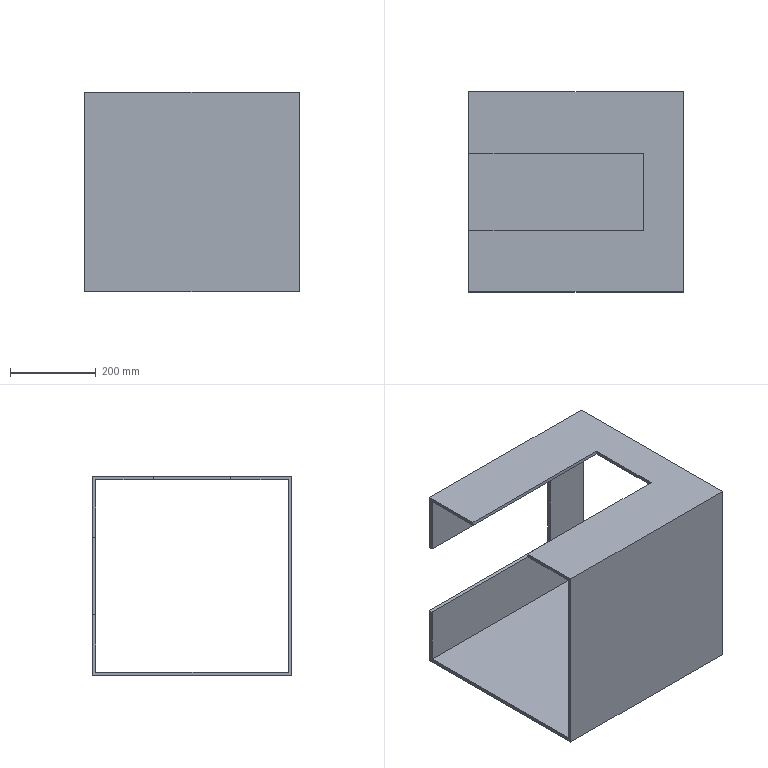Part | SolidWorks | features Cut 2, DeleteBody 1, Extrusion 1, MoveCopyBody 1, Stock 1 | 1 solid | 17 faces | box 500 x 466 x 466 mm | volume 6178880 mm3 | plane 17
STEP:
#1=CARTESIAN_POINT('',(0.,-90.,233.));
#2=VERTEX_POINT('',#1);
#3=CARTESIAN_POINT('',(0.,-233.,233.));
#4=VERTEX_POINT('',#3);
#5=CARTESIAN_POINT('',(0.,233.,233.));
#6=DIRECTION('',(0.,-1.,0.));
#7=VECTOR('',#6,1000.);
#8=LINE('',#5,#7);
#9=EDGE_CURVE('',#2,#4,#8,.T.);
#10=ORIENTED_EDGE('',*,*,#9,.F.);
#11=CARTESIAN_POINT('',(0.,-90.,225.));
#12=VERTEX_POINT('',#11);
#13=CARTESIAN_POINT('',(0.,-90.,98.286));
#14=DIRECTION('',(0.,0.,1.));
#15=VECTOR('',#14,1000.);
#16=LINE('',#13,#15);
#17=EDGE_CURVE('',#12,#2,#16,.T.);
#18=ORIENTED_EDGE('',*,*,#17,.F.);
#19=CARTESIAN_POINT('',(0.,-225.,225.));
#20=VERTEX_POINT('',#19);
#21=CARTESIAN_POINT('',(0.,225.,225.));
#22=DIRECTION('',(0.,-1.,0.));
#23=VECTOR('',#22,1000.);
#24=LINE('',#21,#23);
#25=EDGE_CURVE('',#12,#20,#24,.T.);
#26=ORIENTED_EDGE('',*,*,#25,.T.);
#27=CARTESIAN_POINT('',(0.,-225.,-225.));
#28=VERTEX_POINT('',#27);
#29=CARTESIAN_POINT('',(0.,-225.,225.));
#30=DIRECTION('',(0.,0.,-1.));
#31=VECTOR('',#30,1000.);
#32=LINE('',#29,#31);
#33=EDGE_CURVE('',#20,#28,#32,.T.);
#34=ORIENTED_EDGE('',*,*,#33,.T.);
#35=CARTESIAN_POINT('',(0.,225.,-225.));
#36=VERTEX_POINT('',#35);
#37=CARTESIAN_POINT('',(0.,225.,-225.));
#38=DIRECTION('',(0.,1.,0.));
#39=VECTOR('',#38,1000.);
#40=LINE('',#37,#39);
#41=EDGE_CURVE('',#28,#36,#40,.T.);
#42=ORIENTED_EDGE('',*,*,#41,.T.);
#43=CARTESIAN_POINT('',(0.,225.,-90.));
#44=VERTEX_POINT('',#43);
#45=CARTESIAN_POINT('',(0.,225.,225.));
#46=DIRECTION('',(0.,0.,1.));
#47=VECTOR('',#46,1000.);
#48=LINE('',#45,#47);
#49=EDGE_CURVE('',#36,#44,#48,.T.);
#50=ORIENTED_EDGE('',*,*,#49,.T.);
#51=CARTESIAN_POINT('',(0.,233.,-90.));
#52=VERTEX_POINT('',#51);
#53=CARTESIAN_POINT('',(0.,0.,-90.));
#54=DIRECTION('',(0.,1.,0.));
#55=VECTOR('',#54,1000.);
#56=LINE('',#53,#55);
#57=EDGE_CURVE('',#44,#52,#56,.T.);
#58=ORIENTED_EDGE('',*,*,#57,.T.);
#59=CARTESIAN_POINT('',(0.,233.,-233.));
#60=VERTEX_POINT('',#59);
#61=CARTESIAN_POINT('',(0.,233.,233.));
#62=DIRECTION('',(0.,0.,1.));
#63=VECTOR('',#62,1000.);
#64=LINE('',#61,#63);
#65=EDGE_CURVE('',#60,#52,#64,.T.);
#66=ORIENTED_EDGE('',*,*,#65,.F.);
#67=CARTESIAN_POINT('',(0.,-233.,-233.));
#68=VERTEX_POINT('',#67);
#69=CARTESIAN_POINT('',(0.,233.,-233.));
#70=DIRECTION('',(0.,1.,0.));
#71=VECTOR('',#70,1000.);
#72=LINE('',#69,#71);
#73=EDGE_CURVE('',#68,#60,#72,.T.);
#74=ORIENTED_EDGE('',*,*,#73,.F.);
#75=CARTESIAN_POINT('',(0.,-233.,233.));
#76=DIRECTION('',(0.,0.,-1.));
#77=VECTOR('',#76,1000.);
#78=LINE('',#75,#77);
#79=EDGE_CURVE('',#4,#68,#78,.T.);
#80=ORIENTED_EDGE('',*,*,#79,.F.);
#81=EDGE_LOOP('',(#10,#18,#26,#34,#42,#50,#58,#66,#74,#80));
#82=FACE_OUTER_BOUND('',#81,.T.);
#83=CARTESIAN_POINT('',(0.,0.,0.));
#84=DIRECTION('',(1.,0.,0.));
#85=DIRECTION('',(0.,0.,-1.));
#86=AXIS2_PLACEMENT_3D('',#83,#84,#85);
#87=PLANE('',#86);
#88=ADVANCED_FACE('',(#82),#87,.F.);
#89=CARTESIAN_POINT('',(500.,-233.,-233.));
#90=VERTEX_POINT('',#89);
#91=CARTESIAN_POINT('',(500.,233.,-233.));
#92=VERTEX_POINT('',#91);
#93=CARTESIAN_POINT('',(500.,233.,-233.));
#94=DIRECTION('',(0.,1.,0.));
#95=VECTOR('',#94,1000.);
#96=LINE('',#93,#95);
#97=EDGE_CURVE('',#90,#92,#96,.T.);
#98=ORIENTED_EDGE('',*,*,#97,.T.);
#99=CARTESIAN_POINT('',(500.,233.,233.));
#100=VERTEX_POINT('',#99);
#101=CARTESIAN_POINT('',(500.,233.,233.));
#102=DIRECTION('',(0.,0.,1.));
#103=VECTOR('',#102,1000.);
#104=LINE('',#101,#103);
#105=EDGE_CURVE('',#92,#100,#104,.T.);
#106=ORIENTED_EDGE('',*,*,#105,.T.);
#107=CARTESIAN_POINT('',(500.,-233.,233.));
#108=VERTEX_POINT('',#107);
#109=CARTESIAN_POINT('',(500.,233.,233.));
#110=DIRECTION('',(0.,-1.,0.));
#111=VECTOR('',#110,1000.);
#112=LINE('',#109,#111);
#113=EDGE_CURVE('',#100,#108,#112,.T.);
#114=ORIENTED_EDGE('',*,*,#113,.T.);
#115=CARTESIAN_POINT('',(500.,-233.,233.));
#116=DIRECTION('',(0.,0.,-1.));
#117=VECTOR('',#116,1000.);
#118=LINE('',#115,#117);
#119=EDGE_CURVE('',#108,#90,#118,.T.);
#120=ORIENTED_EDGE('',*,*,#119,.T.);
#121=EDGE_LOOP('',(#98,#106,#114,#120));
#122=FACE_OUTER_BOUND('',#121,.T.);
#123=CARTESIAN_POINT('',(500.,225.,-225.));
#124=VERTEX_POINT('',#123);
#125=CARTESIAN_POINT('',(500.,225.,225.));
#126=VERTEX_POINT('',#125);
#127=CARTESIAN_POINT('',(500.,225.,225.));
#128=DIRECTION('',(0.,0.,1.));
#129=VECTOR('',#128,1000.);
#130=LINE('',#127,#129);
#131=EDGE_CURVE('',#124,#126,#130,.T.);
#132=ORIENTED_EDGE('',*,*,#131,.F.);
#133=CARTESIAN_POINT('',(500.,-225.,-225.));
#134=VERTEX_POINT('',#133);
#135=CARTESIAN_POINT('',(500.,225.,-225.));
#136=DIRECTION('',(0.,1.,0.));
#137=VECTOR('',#136,1000.);
#138=LINE('',#135,#137);
#139=EDGE_CURVE('',#134,#124,#138,.T.);
#140=ORIENTED_EDGE('',*,*,#139,.F.);
#141=CARTESIAN_POINT('',(500.,-225.,225.));
#142=VERTEX_POINT('',#141);
#143=CARTESIAN_POINT('',(500.,-225.,225.));
#144=DIRECTION('',(0.,0.,-1.));
#145=VECTOR('',#144,1000.);
#146=LINE('',#143,#145);
#147=EDGE_CURVE('',#142,#134,#146,.T.);
#148=ORIENTED_EDGE('',*,*,#147,.F.);
#149=CARTESIAN_POINT('',(500.,225.,225.));
#150=DIRECTION('',(0.,-1.,0.));
#151=VECTOR('',#150,1000.);
#152=LINE('',#149,#151);
#153=EDGE_CURVE('',#126,#142,#152,.T.);
#154=ORIENTED_EDGE('',*,*,#153,.F.);
#155=EDGE_LOOP('',(#132,#140,#148,#154));
#156=FACE_BOUND('',#155,.T.);
#157=CARTESIAN_POINT('',(500.,0.,0.));
#158=DIRECTION('',(1.,0.,0.));
#159=DIRECTION('',(0.,0.,-1.));
#160=AXIS2_PLACEMENT_3D('',#157,#158,#159);
#161=PLANE('',#160);
#162=ADVANCED_FACE('',(#122,#156),#161,.T.);
#163=CARTESIAN_POINT('',(0.,225.,225.));
#164=VERTEX_POINT('',#163);
#165=CARTESIAN_POINT('',(0.,90.,225.));
#166=VERTEX_POINT('',#165);
#167=CARTESIAN_POINT('',(0.,225.,225.));
#168=DIRECTION('',(0.,-1.,0.));
#169=VECTOR('',#168,1000.);
#170=LINE('',#167,#169);
#171=EDGE_CURVE('',#164,#166,#170,.T.);
#172=ORIENTED_EDGE('',*,*,#171,.T.);
#173=CARTESIAN_POINT('',(0.,90.,233.));
#174=VERTEX_POINT('',#173);
#175=CARTESIAN_POINT('',(0.,90.,98.286));
#176=DIRECTION('',(0.,0.,-1.));
#177=VECTOR('',#176,1000.);
#178=LINE('',#175,#177);
#179=EDGE_CURVE('',#174,#166,#178,.T.);
#180=ORIENTED_EDGE('',*,*,#179,.F.);
#181=CARTESIAN_POINT('',(0.,233.,233.));
#182=VERTEX_POINT('',#181);
#183=CARTESIAN_POINT('',(0.,233.,233.));
#184=DIRECTION('',(0.,-1.,0.));
#185=VECTOR('',#184,1000.);
#186=LINE('',#183,#185);
#187=EDGE_CURVE('',#182,#174,#186,.T.);
#188=ORIENTED_EDGE('',*,*,#187,.F.);
#189=CARTESIAN_POINT('',(0.,233.,90.));
#190=VERTEX_POINT('',#189);
#191=CARTESIAN_POINT('',(0.,233.,233.));
#192=DIRECTION('',(0.,0.,1.));
#193=VECTOR('',#192,1000.);
#194=LINE('',#191,#193);
#195=EDGE_CURVE('',#190,#182,#194,.T.);
#196=ORIENTED_EDGE('',*,*,#195,.F.);
#197=CARTESIAN_POINT('',(0.,225.,90.));
#198=VERTEX_POINT('',#197);
#199=CARTESIAN_POINT('',(0.,0.,90.));
#200=DIRECTION('',(0.,-1.,0.));
#201=VECTOR('',#200,1000.);
#202=LINE('',#199,#201);
#203=EDGE_CURVE('',#190,#198,#202,.T.);
#204=ORIENTED_EDGE('',*,*,#203,.T.);
#205=CARTESIAN_POINT('',(0.,225.,225.));
#206=DIRECTION('',(0.,0.,1.));
#207=VECTOR('',#206,1000.);
#208=LINE('',#205,#207);
#209=EDGE_CURVE('',#198,#164,#208,.T.);
#210=ORIENTED_EDGE('',*,*,#209,.T.);
#211=EDGE_LOOP('',(#172,#180,#188,#196,#204,#210));
#212=FACE_OUTER_BOUND('',#211,.T.);
#213=CARTESIAN_POINT('',(0.,0.,0.));
#214=DIRECTION('',(1.,0.,0.));
#215=DIRECTION('',(0.,0.,-1.));
#216=AXIS2_PLACEMENT_3D('',#213,#214,#215);
#217=PLANE('',#216);
#218=ADVANCED_FACE('',(#212),#217,.F.);
#219=ORIENTED_EDGE('',*,*,#73,.T.);
#220=CARTESIAN_POINT('',(500.,233.,-233.));
#221=DIRECTION('',(-1.,0.,0.));
#222=VECTOR('',#221,1000.);
#223=LINE('',#220,#222);
#224=EDGE_CURVE('',#92,#60,#223,.T.);
#225=ORIENTED_EDGE('',*,*,#224,.F.);
#226=ORIENTED_EDGE('',*,*,#97,.F.);
#227=CARTESIAN_POINT('',(500.,-233.,-233.));
#228=DIRECTION('',(-1.,0.,0.));
#229=VECTOR('',#228,1000.);
#230=LINE('',#227,#229);
#231=EDGE_CURVE('',#90,#68,#230,.T.);
#232=ORIENTED_EDGE('',*,*,#231,.T.);
#233=EDGE_LOOP('',(#219,#225,#226,#232));
#234=FACE_OUTER_BOUND('',#233,.T.);
#235=CARTESIAN_POINT('',(500.,233.,-233.));
#236=DIRECTION('',(0.,0.,1.));
#237=DIRECTION('',(0.,-1.,0.));
#238=AXIS2_PLACEMENT_3D('',#235,#236,#237);
#239=PLANE('',#238);
#240=ADVANCED_FACE('',(#234),#239,.F.);
#241=CARTESIAN_POINT('',(390.,233.,90.));
#242=VERTEX_POINT('',#241);
#243=CARTESIAN_POINT('',(390.,233.,-90.));
#244=VERTEX_POINT('',#243);
#245=CARTESIAN_POINT('',(390.,233.,-90.));
#246=DIRECTION('',(0.,0.,-1.));
#247=VECTOR('',#246,1000.);
#248=LINE('',#245,#247);
#249=EDGE_CURVE('',#242,#244,#248,.T.);
#250=ORIENTED_EDGE('',*,*,#249,.F.);
#251=CARTESIAN_POINT('',(-390.,233.,90.));
#252=DIRECTION('',(1.,0.,0.));
#253=VECTOR('',#252,1000.);
#254=LINE('',#251,#253);
#255=EDGE_CURVE('',#190,#242,#254,.T.);
#256=ORIENTED_EDGE('',*,*,#255,.F.);
#257=ORIENTED_EDGE('',*,*,#195,.T.);
#258=CARTESIAN_POINT('',(500.,233.,233.));
#259=DIRECTION('',(-1.,0.,0.));
#260=VECTOR('',#259,1000.);
#261=LINE('',#258,#260);
#262=EDGE_CURVE('',#100,#182,#261,.T.);
#263=ORIENTED_EDGE('',*,*,#262,.F.);
#264=ORIENTED_EDGE('',*,*,#105,.F.);
#265=ORIENTED_EDGE('',*,*,#224,.T.);
#266=ORIENTED_EDGE('',*,*,#65,.T.);
#267=CARTESIAN_POINT('',(-390.,233.,-90.));
#268=DIRECTION('',(-1.,0.,0.));
#269=VECTOR('',#268,1000.);
#270=LINE('',#267,#269);
#271=EDGE_CURVE('',#244,#52,#270,.T.);
#272=ORIENTED_EDGE('',*,*,#271,.F.);
#273=EDGE_LOOP('',(#250,#256,#257,#263,#264,#265,#266,#272));
#274=FACE_OUTER_BOUND('',#273,.T.);
#275=CARTESIAN_POINT('',(500.,233.,233.));
#276=DIRECTION('',(0.,-1.,0.));
#277=DIRECTION('',(0.,0.,-1.));
#278=AXIS2_PLACEMENT_3D('',#275,#276,#277);
#279=PLANE('',#278);
#280=ADVANCED_FACE('',(#274),#279,.F.);
#281=CARTESIAN_POINT('',(408.,-90.,233.));
#282=VERTEX_POINT('',#281);
#283=CARTESIAN_POINT('',(408.,90.,233.));
#284=VERTEX_POINT('',#283);
#285=CARTESIAN_POINT('',(408.,233.,233.));
#286=DIRECTION('',(0.,1.,0.));
#287=VECTOR('',#286,1000.);
#288=LINE('',#285,#287);
#289=EDGE_CURVE('',#282,#284,#288,.T.);
#290=ORIENTED_EDGE('',*,*,#289,.F.);
#291=CARTESIAN_POINT('',(500.,-90.,233.));
#292=DIRECTION('',(-1.,0.,0.));
#293=VECTOR('',#292,1000.);
#294=LINE('',#291,#293);
#295=EDGE_CURVE('',#282,#2,#294,.T.);
#296=ORIENTED_EDGE('',*,*,#295,.T.);
#297=ORIENTED_EDGE('',*,*,#9,.T.);
#298=CARTESIAN_POINT('',(500.,-233.,233.));
#299=DIRECTION('',(-1.,0.,0.));
#300=VECTOR('',#299,1000.);
#301=LINE('',#298,#300);
#302=EDGE_CURVE('',#108,#4,#301,.T.);
#303=ORIENTED_EDGE('',*,*,#302,.F.);
#304=ORIENTED_EDGE('',*,*,#113,.F.);
#305=ORIENTED_EDGE('',*,*,#262,.T.);
#306=ORIENTED_EDGE('',*,*,#187,.T.);
#307=CARTESIAN_POINT('',(500.,90.,233.));
#308=DIRECTION('',(1.,0.,0.));
#309=VECTOR('',#308,1000.);
#310=LINE('',#307,#309);
#311=EDGE_CURVE('',#174,#284,#310,.T.);
#312=ORIENTED_EDGE('',*,*,#311,.T.);
#313=EDGE_LOOP('',(#290,#296,#297,#303,#304,#305,#306,#312));
#314=FACE_OUTER_BOUND('',#313,.T.);
#315=CARTESIAN_POINT('',(500.,233.,233.));
#316=DIRECTION('',(0.,0.,-1.));
#317=DIRECTION('',(0.,1.,0.));
#318=AXIS2_PLACEMENT_3D('',#315,#316,#317);
#319=PLANE('',#318);
#320=ADVANCED_FACE('',(#314),#319,.F.);
#321=ORIENTED_EDGE('',*,*,#79,.T.);
#322=ORIENTED_EDGE('',*,*,#231,.F.);
#323=ORIENTED_EDGE('',*,*,#119,.F.);
#324=ORIENTED_EDGE('',*,*,#302,.T.);
#325=EDGE_LOOP('',(#321,#322,#323,#324));
#326=FACE_OUTER_BOUND('',#325,.T.);
#327=CARTESIAN_POINT('',(500.,-233.,233.));
#328=DIRECTION('',(0.,1.,0.));
#329=DIRECTION('',(0.,0.,1.));
#330=AXIS2_PLACEMENT_3D('',#327,#328,#329);
#331=PLANE('',#330);
#332=ADVANCED_FACE('',(#326),#331,.F.);
#333=ORIENTED_EDGE('',*,*,#41,.F.);
#334=CARTESIAN_POINT('',(500.,-225.,-225.));
#335=DIRECTION('',(-1.,0.,0.));
#336=VECTOR('',#335,1000.);
#337=LINE('',#334,#336);
#338=EDGE_CURVE('',#134,#28,#337,.T.);
#339=ORIENTED_EDGE('',*,*,#338,.F.);
#340=ORIENTED_EDGE('',*,*,#139,.T.);
#341=CARTESIAN_POINT('',(500.,225.,-225.));
#342=DIRECTION('',(-1.,0.,0.));
#343=VECTOR('',#342,1000.);
#344=LINE('',#341,#343);
#345=EDGE_CURVE('',#124,#36,#344,.T.);
#346=ORIENTED_EDGE('',*,*,#345,.T.);
#347=EDGE_LOOP('',(#333,#339,#340,#346));
#348=FACE_OUTER_BOUND('',#347,.T.);
#349=CARTESIAN_POINT('',(500.,225.,-225.));
#350=DIRECTION('',(0.,0.,1.));
#351=DIRECTION('',(0.,-1.,0.));
#352=AXIS2_PLACEMENT_3D('',#349,#350,#351);
#353=PLANE('',#352);
#354=ADVANCED_FACE('',(#348),#353,.T.);
#355=CARTESIAN_POINT('',(390.,225.,90.));
#356=VERTEX_POINT('',#355);
#357=CARTESIAN_POINT('',(500.,225.,90.));
#358=DIRECTION('',(-1.,0.,0.));
#359=VECTOR('',#358,1000.);
#360=LINE('',#357,#359);
#361=EDGE_CURVE('',#356,#198,#360,.T.);
#362=ORIENTED_EDGE('',*,*,#361,.F.);
#363=CARTESIAN_POINT('',(390.,225.,-90.));
#364=VERTEX_POINT('',#363);
#365=CARTESIAN_POINT('',(390.,225.,225.));
#366=DIRECTION('',(0.,0.,1.));
#367=VECTOR('',#366,1000.);
#368=LINE('',#365,#367);
#369=EDGE_CURVE('',#364,#356,#368,.T.);
#370=ORIENTED_EDGE('',*,*,#369,.F.);
#371=CARTESIAN_POINT('',(500.,225.,-90.));
#372=DIRECTION('',(1.,0.,0.));
#373=VECTOR('',#372,1000.);
#374=LINE('',#371,#373);
#375=EDGE_CURVE('',#44,#364,#374,.T.);
#376=ORIENTED_EDGE('',*,*,#375,.F.);
#377=ORIENTED_EDGE('',*,*,#49,.F.);
#378=ORIENTED_EDGE('',*,*,#345,.F.);
#379=ORIENTED_EDGE('',*,*,#131,.T.);
#380=CARTESIAN_POINT('',(500.,225.,225.));
#381=DIRECTION('',(-1.,0.,0.));
#382=VECTOR('',#381,1000.);
#383=LINE('',#380,#382);
#384=EDGE_CURVE('',#126,#164,#383,.T.);
#385=ORIENTED_EDGE('',*,*,#384,.T.);
#386=ORIENTED_EDGE('',*,*,#209,.F.);
#387=EDGE_LOOP('',(#362,#370,#376,#377,#378,#379,#385,#386));
#388=FACE_OUTER_BOUND('',#387,.T.);
#389=CARTESIAN_POINT('',(500.,225.,225.));
#390=DIRECTION('',(0.,-1.,0.));
#391=DIRECTION('',(0.,0.,-1.));
#392=AXIS2_PLACEMENT_3D('',#389,#390,#391);
#393=PLANE('',#392);
#394=ADVANCED_FACE('',(#388),#393,.T.);
#395=CARTESIAN_POINT('',(408.,-90.,225.));
#396=VERTEX_POINT('',#395);
#397=CARTESIAN_POINT('',(500.,-90.,225.));
#398=DIRECTION('',(-1.,0.,0.));
#399=VECTOR('',#398,1000.);
#400=LINE('',#397,#399);
#401=EDGE_CURVE('',#396,#12,#400,.T.);
#402=ORIENTED_EDGE('',*,*,#401,.F.);
#403=CARTESIAN_POINT('',(408.,90.,225.));
#404=VERTEX_POINT('',#403);
#405=CARTESIAN_POINT('',(408.,225.,225.));
#406=DIRECTION('',(0.,1.,0.));
#407=VECTOR('',#406,1000.);
#408=LINE('',#405,#407);
#409=EDGE_CURVE('',#396,#404,#408,.T.);
#410=ORIENTED_EDGE('',*,*,#409,.T.);
#411=CARTESIAN_POINT('',(500.,90.,225.));
#412=DIRECTION('',(1.,0.,0.));
#413=VECTOR('',#412,1000.);
#414=LINE('',#411,#413);
#415=EDGE_CURVE('',#166,#404,#414,.T.);
#416=ORIENTED_EDGE('',*,*,#415,.F.);
#417=ORIENTED_EDGE('',*,*,#171,.F.);
#418=ORIENTED_EDGE('',*,*,#384,.F.);
#419=ORIENTED_EDGE('',*,*,#153,.T.);
#420=CARTESIAN_POINT('',(500.,-225.,225.));
#421=DIRECTION('',(-1.,0.,0.));
#422=VECTOR('',#421,1000.);
#423=LINE('',#420,#422);
#424=EDGE_CURVE('',#142,#20,#423,.T.);
#425=ORIENTED_EDGE('',*,*,#424,.T.);
#426=ORIENTED_EDGE('',*,*,#25,.F.);
#427=EDGE_LOOP('',(#402,#410,#416,#417,#418,#419,#425,#426));
#428=FACE_OUTER_BOUND('',#427,.T.);
#429=CARTESIAN_POINT('',(500.,225.,225.));
#430=DIRECTION('',(0.,0.,-1.));
#431=DIRECTION('',(0.,1.,0.));
#432=AXIS2_PLACEMENT_3D('',#429,#430,#431);
#433=PLANE('',#432);
#434=ADVANCED_FACE('',(#428),#433,.T.);
#435=ORIENTED_EDGE('',*,*,#33,.F.);
#436=ORIENTED_EDGE('',*,*,#424,.F.);
#437=ORIENTED_EDGE('',*,*,#147,.T.);
#438=ORIENTED_EDGE('',*,*,#338,.T.);
#439=EDGE_LOOP('',(#435,#436,#437,#438));
#440=FACE_OUTER_BOUND('',#439,.T.);
#441=CARTESIAN_POINT('',(500.,-225.,225.));
#442=DIRECTION('',(0.,1.,0.));
#443=DIRECTION('',(0.,0.,1.));
#444=AXIS2_PLACEMENT_3D('',#441,#442,#443);
#445=PLANE('',#444);
#446=ADVANCED_FACE('',(#440),#445,.T.);
#447=ORIENTED_EDGE('',*,*,#255,.T.);
#448=CARTESIAN_POINT('',(390.,-175.,90.));
#449=DIRECTION('',(0.,1.,0.));
#450=VECTOR('',#449,1000.);
#451=LINE('',#448,#450);
#452=EDGE_CURVE('',#356,#242,#451,.T.);
#453=ORIENTED_EDGE('',*,*,#452,.F.);
#454=ORIENTED_EDGE('',*,*,#361,.T.);
#455=ORIENTED_EDGE('',*,*,#203,.F.);
#456=EDGE_LOOP('',(#447,#453,#454,#455));
#457=FACE_OUTER_BOUND('',#456,.T.);
#458=CARTESIAN_POINT('',(-390.,-175.,90.));
#459=DIRECTION('',(0.,0.,1.));
#460=DIRECTION('',(1.,0.,0.));
#461=AXIS2_PLACEMENT_3D('',#458,#459,#460);
#462=PLANE('',#461);
#463=ADVANCED_FACE('',(#457),#462,.F.);
#464=ORIENTED_EDGE('',*,*,#375,.T.);
#465=CARTESIAN_POINT('',(390.,-175.,-90.));
#466=DIRECTION('',(0.,1.,0.));
#467=VECTOR('',#466,1000.);
#468=LINE('',#465,#467);
#469=EDGE_CURVE('',#364,#244,#468,.T.);
#470=ORIENTED_EDGE('',*,*,#469,.T.);
#471=ORIENTED_EDGE('',*,*,#271,.T.);
#472=ORIENTED_EDGE('',*,*,#57,.F.);
#473=EDGE_LOOP('',(#464,#470,#471,#472));
#474=FACE_OUTER_BOUND('',#473,.T.);
#475=CARTESIAN_POINT('',(-390.,-175.,-90.));
#476=DIRECTION('',(0.,0.,-1.));
#477=DIRECTION('',(-1.,0.,0.));
#478=AXIS2_PLACEMENT_3D('',#475,#476,#477);
#479=PLANE('',#478);
#480=ADVANCED_FACE('',(#474),#479,.F.);
#481=ORIENTED_EDGE('',*,*,#369,.T.);
#482=ORIENTED_EDGE('',*,*,#452,.T.);
#483=ORIENTED_EDGE('',*,*,#249,.T.);
#484=ORIENTED_EDGE('',*,*,#469,.F.);
#485=EDGE_LOOP('',(#481,#482,#483,#484));
#486=FACE_OUTER_BOUND('',#485,.T.);
#487=CARTESIAN_POINT('',(390.,-175.,-90.));
#488=DIRECTION('',(1.,0.,0.));
#489=DIRECTION('',(0.,0.,-1.));
#490=AXIS2_PLACEMENT_3D('',#487,#488,#489);
#491=PLANE('',#490);
#492=ADVANCED_FACE('',(#486),#491,.F.);
#493=CARTESIAN_POINT('',(408.,-90.,98.286));
#494=DIRECTION('',(0.,0.,1.));
#495=VECTOR('',#494,1000.);
#496=LINE('',#493,#495);
#497=EDGE_CURVE('',#396,#282,#496,.T.);
#498=ORIENTED_EDGE('',*,*,#497,.F.);
#499=ORIENTED_EDGE('',*,*,#401,.T.);
#500=ORIENTED_EDGE('',*,*,#17,.T.);
#501=ORIENTED_EDGE('',*,*,#295,.F.);
#502=EDGE_LOOP('',(#498,#499,#500,#501));
#503=FACE_OUTER_BOUND('',#502,.T.);
#504=CARTESIAN_POINT('',(408.,-90.,98.286));
#505=DIRECTION('',(0.,-1.,0.));
#506=DIRECTION('',(0.,0.,-1.));
#507=AXIS2_PLACEMENT_3D('',#504,#505,#506);
#508=PLANE('',#507);
#509=ADVANCED_FACE('',(#503),#508,.F.);
#510=ORIENTED_EDGE('',*,*,#179,.T.);
#511=ORIENTED_EDGE('',*,*,#415,.T.);
#512=CARTESIAN_POINT('',(408.,90.,98.286));
#513=DIRECTION('',(0.,0.,-1.));
#514=VECTOR('',#513,1000.);
#515=LINE('',#512,#514);
#516=EDGE_CURVE('',#284,#404,#515,.T.);
#517=ORIENTED_EDGE('',*,*,#516,.F.);
#518=ORIENTED_EDGE('',*,*,#311,.F.);
#519=EDGE_LOOP('',(#510,#511,#517,#518));
#520=FACE_OUTER_BOUND('',#519,.T.);
#521=CARTESIAN_POINT('',(408.,90.,98.286));
#522=DIRECTION('',(0.,1.,0.));
#523=DIRECTION('',(0.,0.,1.));
#524=AXIS2_PLACEMENT_3D('',#521,#522,#523);
#525=PLANE('',#524);
#526=ADVANCED_FACE('',(#520),#525,.F.);
#527=ORIENTED_EDGE('',*,*,#289,.T.);
#528=ORIENTED_EDGE('',*,*,#516,.T.);
#529=ORIENTED_EDGE('',*,*,#409,.F.);
#530=ORIENTED_EDGE('',*,*,#497,.T.);
#531=EDGE_LOOP('',(#527,#528,#529,#530));
#532=FACE_OUTER_BOUND('',#531,.T.);
#533=CARTESIAN_POINT('',(408.,0.,0.));
#534=DIRECTION('',(-1.,0.,0.));
#535=DIRECTION('',(0.,0.,1.));
#536=AXIS2_PLACEMENT_3D('',#533,#534,#535);
#537=PLANE('',#536);
#538=ADVANCED_FACE('',(#532),#537,.T.);
#539=CLOSED_SHELL('',(#88,#162,#218,#240,#280,#320,#332,#354,#394,#434,#446,#463,#480,#492,#509,#526,#538));
#540=MANIFOLD_SOLID_BREP('',#539);
#541=CARTESIAN_POINT('',(0.,0.,0.));
#542=DIRECTION('',(0.,0.,1.));
#543=DIRECTION('',(1.,0.,0.));
#544=AXIS2_PLACEMENT_3D('',#541,#542,#543);
#545=(LENGTH_UNIT()NAMED_UNIT(*)SI_UNIT(.MILLI.,.METRE.));
#546=UNCERTAINTY_MEASURE_WITH_UNIT(LENGTH_MEASURE(0.00001),#545,'','');
#547=(NAMED_UNIT(*)PLANE_ANGLE_UNIT()SI_UNIT($,.RADIAN.));
#548=(NAMED_UNIT(*)SI_UNIT($,.STERADIAN.)SOLID_ANGLE_UNIT());
#549=(GEOMETRIC_REPRESENTATION_CONTEXT(3)GLOBAL_UNCERTAINTY_ASSIGNED_CONTEXT((#546))GLOBAL_UNIT_ASSIGNED_CONTEXT((#545,#547,#548))REPRESENTATION_CONTEXT('',''));
#550=ADVANCED_BREP_SHAPE_REPRESENTATION('',(#540,#544),#549);